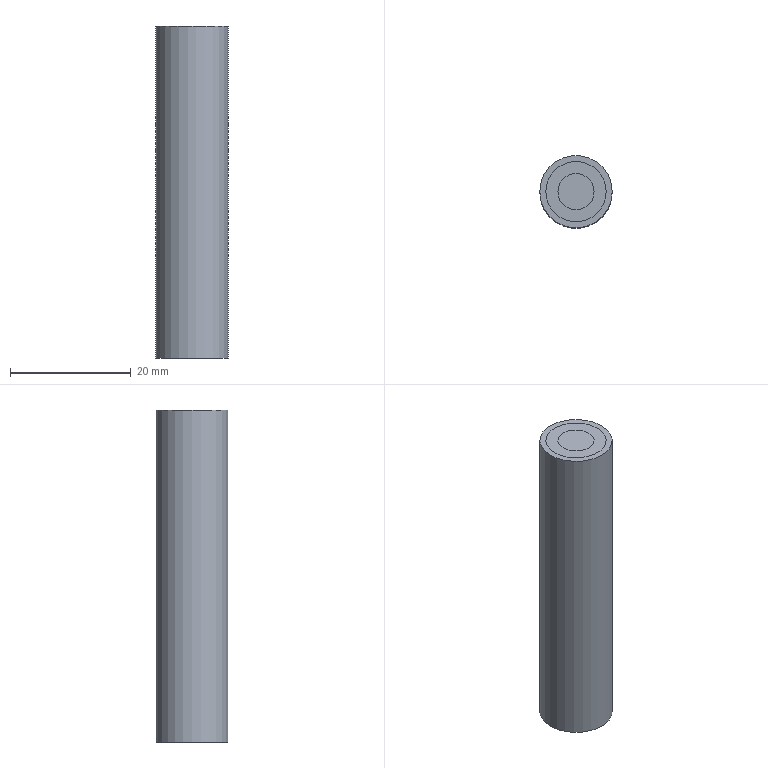Part | NX | features BREP 2 | 2 solids | 7 faces | box 12 x 12 x 55 mm | volume 8985 mm3 | plane 4 | cylinder 3 | commonest cylinder face diameters 6 x1 10 x1 12 x1
STEP:
#1=CARTESIAN_POINT('',(6.,0.,55.));
#2=VERTEX_POINT('',#1);
#3=CARTESIAN_POINT('',(0.,0.,55.));
#4=DIRECTION('',(0.,0.,1.));
#5=DIRECTION('',(1.,0.,0.));
#6=AXIS2_PLACEMENT_3D('',#3,#4,#5);
#7=CIRCLE('',#6,6.);
#8=EDGE_CURVE('',#2,#2,#7,.T.);
#9=ORIENTED_EDGE('',*,*,#8,.F.);
#10=EDGE_LOOP('',(#9));
#11=FACE_BOUND('',#10,.T.);
#12=CARTESIAN_POINT('',(6.,0.,0.));
#13=VERTEX_POINT('',#12);
#14=CARTESIAN_POINT('',(0.,0.,0.));
#15=DIRECTION('',(0.,0.,1.));
#16=DIRECTION('',(1.,0.,0.));
#17=AXIS2_PLACEMENT_3D('',#14,#15,#16);
#18=CIRCLE('',#17,6.);
#19=EDGE_CURVE('',#13,#13,#18,.T.);
#20=ORIENTED_EDGE('',*,*,#19,.T.);
#21=EDGE_LOOP('',(#20));
#22=FACE_BOUND('',#21,.T.);
#23=CARTESIAN_POINT('',(0.,0.,55.));
#24=DIRECTION('',(0.,0.,-1.));
#25=DIRECTION('',(1.,0.,0.));
#26=AXIS2_PLACEMENT_3D('',#23,#24,#25);
#27=CYLINDRICAL_SURFACE('',#26,6.);
#28=ADVANCED_FACE('',(#11,#22),#27,.T.);
#29=ORIENTED_EDGE('',*,*,#8,.T.);
#30=EDGE_LOOP('',(#29));
#31=FACE_BOUND('',#30,.T.);
#32=CARTESIAN_POINT('',(0.,0.,55.));
#33=DIRECTION('',(0.,0.,1.));
#34=DIRECTION('',(-1.,0.,0.));
#35=AXIS2_PLACEMENT_3D('',#32,#33,#34);
#36=PLANE('',#35);
#37=ADVANCED_FACE('',(#31),#36,.T.);
#38=ORIENTED_EDGE('',*,*,#19,.F.);
#39=EDGE_LOOP('',(#38));
#40=FACE_BOUND('',#39,.T.);
#41=CARTESIAN_POINT('',(0.,0.,0.));
#42=DIRECTION('',(0.,0.,1.));
#43=DIRECTION('',(-1.,0.,0.));
#44=AXIS2_PLACEMENT_3D('',#41,#42,#43);
#45=PLANE('',#44);
#46=ADVANCED_FACE('',(#40),#45,.F.);
#47=CLOSED_SHELL('',(#28,#37,#46));
#48=MANIFOLD_SOLID_BREP('',#47);
#49=CARTESIAN_POINT('',(5.,0.,55.));
#50=VERTEX_POINT('',#49);
#51=CARTESIAN_POINT('',(0.,0.,55.));
#52=DIRECTION('',(0.,0.,1.));
#53=DIRECTION('',(1.,0.,0.));
#54=AXIS2_PLACEMENT_3D('',#51,#52,#53);
#55=CIRCLE('',#54,5.);
#56=EDGE_CURVE('',#50,#50,#55,.T.);
#57=ORIENTED_EDGE('',*,*,#56,.F.);
#58=EDGE_LOOP('',(#57));
#59=FACE_BOUND('',#58,.T.);
#60=CARTESIAN_POINT('',(5.,0.,0.));
#61=VERTEX_POINT('',#60);
#62=CARTESIAN_POINT('',(0.,0.,0.));
#63=DIRECTION('',(0.,0.,1.));
#64=DIRECTION('',(1.,0.,0.));
#65=AXIS2_PLACEMENT_3D('',#62,#63,#64);
#66=CIRCLE('',#65,5.);
#67=EDGE_CURVE('',#61,#61,#66,.T.);
#68=ORIENTED_EDGE('',*,*,#67,.T.);
#69=EDGE_LOOP('',(#68));
#70=FACE_BOUND('',#69,.T.);
#71=CARTESIAN_POINT('',(0.,0.,55.));
#72=DIRECTION('',(0.,0.,-1.));
#73=DIRECTION('',(1.,0.,0.));
#74=AXIS2_PLACEMENT_3D('',#71,#72,#73);
#75=CYLINDRICAL_SURFACE('',#74,5.);
#76=ADVANCED_FACE('',(#59,#70),#75,.T.);
#77=CARTESIAN_POINT('',(3.,0.,55.));
#78=VERTEX_POINT('',#77);
#79=CARTESIAN_POINT('',(0.,0.,55.));
#80=DIRECTION('',(0.,0.,1.));
#81=DIRECTION('',(1.,0.,0.));
#82=AXIS2_PLACEMENT_3D('',#79,#80,#81);
#83=CIRCLE('',#82,3.);
#84=EDGE_CURVE('',#78,#78,#83,.T.);
#85=ORIENTED_EDGE('',*,*,#84,.T.);
#86=EDGE_LOOP('',(#85));
#87=FACE_BOUND('',#86,.T.);
#88=CARTESIAN_POINT('',(3.,0.,0.));
#89=VERTEX_POINT('',#88);
#90=CARTESIAN_POINT('',(0.,0.,0.));
#91=DIRECTION('',(0.,0.,1.));
#92=DIRECTION('',(1.,0.,0.));
#93=AXIS2_PLACEMENT_3D('',#90,#91,#92);
#94=CIRCLE('',#93,3.);
#95=EDGE_CURVE('',#89,#89,#94,.T.);
#96=ORIENTED_EDGE('',*,*,#95,.F.);
#97=EDGE_LOOP('',(#96));
#98=FACE_BOUND('',#97,.T.);
#99=CARTESIAN_POINT('',(0.,0.,55.));
#100=DIRECTION('',(0.,0.,-1.));
#101=DIRECTION('',(1.,0.,0.));
#102=AXIS2_PLACEMENT_3D('',#99,#100,#101);
#103=CYLINDRICAL_SURFACE('',#102,3.);
#104=ADVANCED_FACE('',(#87,#98),#103,.F.);
#105=ORIENTED_EDGE('',*,*,#56,.T.);
#106=EDGE_LOOP('',(#105));
#107=FACE_BOUND('',#106,.T.);
#108=ORIENTED_EDGE('',*,*,#84,.F.);
#109=EDGE_LOOP('',(#108));
#110=FACE_BOUND('',#109,.T.);
#111=CARTESIAN_POINT('',(0.,0.,55.));
#112=DIRECTION('',(0.,0.,1.));
#113=DIRECTION('',(-1.,0.,0.));
#114=AXIS2_PLACEMENT_3D('',#111,#112,#113);
#115=PLANE('',#114);
#116=ADVANCED_FACE('',(#107,#110),#115,.T.);
#117=ORIENTED_EDGE('',*,*,#67,.F.);
#118=EDGE_LOOP('',(#117));
#119=FACE_BOUND('',#118,.T.);
#120=ORIENTED_EDGE('',*,*,#95,.T.);
#121=EDGE_LOOP('',(#120));
#122=FACE_BOUND('',#121,.T.);
#123=CARTESIAN_POINT('',(0.,0.,0.));
#124=DIRECTION('',(0.,0.,1.));
#125=DIRECTION('',(-1.,0.,0.));
#126=AXIS2_PLACEMENT_3D('',#123,#124,#125);
#127=PLANE('',#126);
#128=ADVANCED_FACE('',(#119,#122),#127,.F.);
#129=CLOSED_SHELL('',(#76,#104,#116,#128));
#130=MANIFOLD_SOLID_BREP('',#129);
#131=(LENGTH_UNIT()NAMED_UNIT(*)SI_UNIT(.MILLI.,.METRE.));
#132=UNCERTAINTY_MEASURE_WITH_UNIT(LENGTH_MEASURE(0.00001),#131,'','');
#133=(NAMED_UNIT(*)PLANE_ANGLE_UNIT()SI_UNIT($,.RADIAN.));
#134=(NAMED_UNIT(*)SI_UNIT($,.STERADIAN.)SOLID_ANGLE_UNIT());
#135=(GEOMETRIC_REPRESENTATION_CONTEXT(3)GLOBAL_UNCERTAINTY_ASSIGNED_CONTEXT((#132))GLOBAL_UNIT_ASSIGNED_CONTEXT((#131,#133,#134))REPRESENTATION_CONTEXT('',''));
#136=ADVANCED_BREP_SHAPE_REPRESENTATION('',(#48,#130),#135);